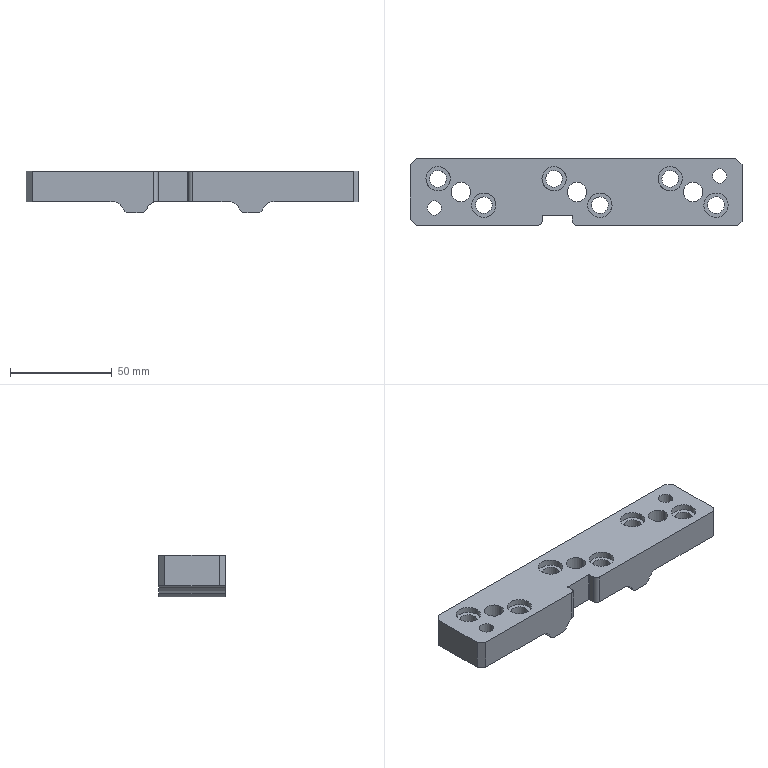Part | STEP file | 1_id1182_x_t | 1 solid | 76 faces | box 163.45 x 32.752 x 20.644 mm | volume 72190 mm3 | cylinder 50 | plane 26 | commonest cylinder face diameters 12 x20 8.2 x12 9.52 x6 5.85 x4 7 x4 0.6 x2